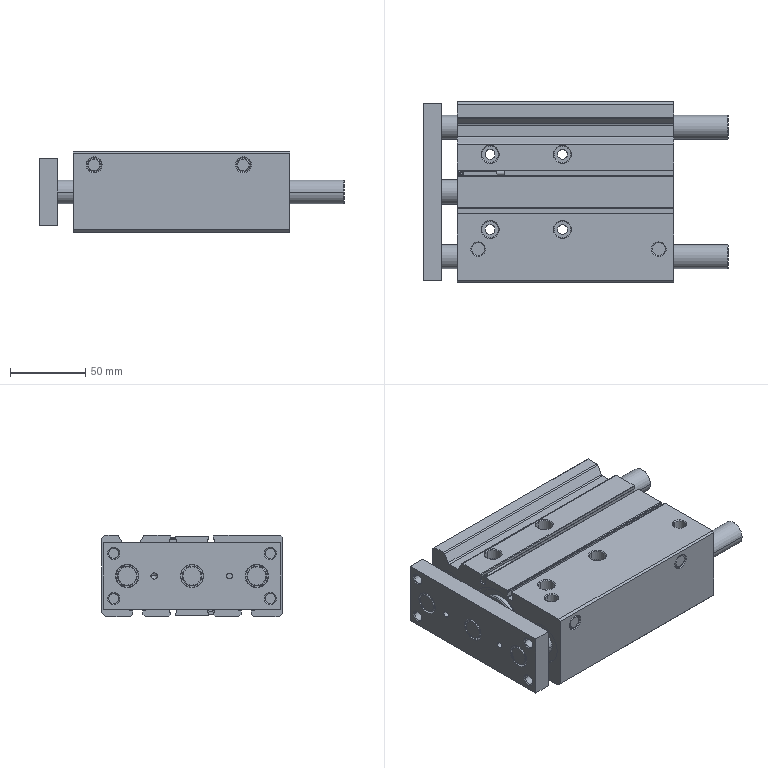Part | NX | features BREP 3 | 4 solids | 446 faces | box 202 x 120 x 54 mm | volume 800850 mm3 | cylinder 191 | plane 153 | cone 92 | torus 10 | commonest cylinder face diameters 0.8 x28 6.647 x24 4 x21 0.4 x16 16 x12 2 x8